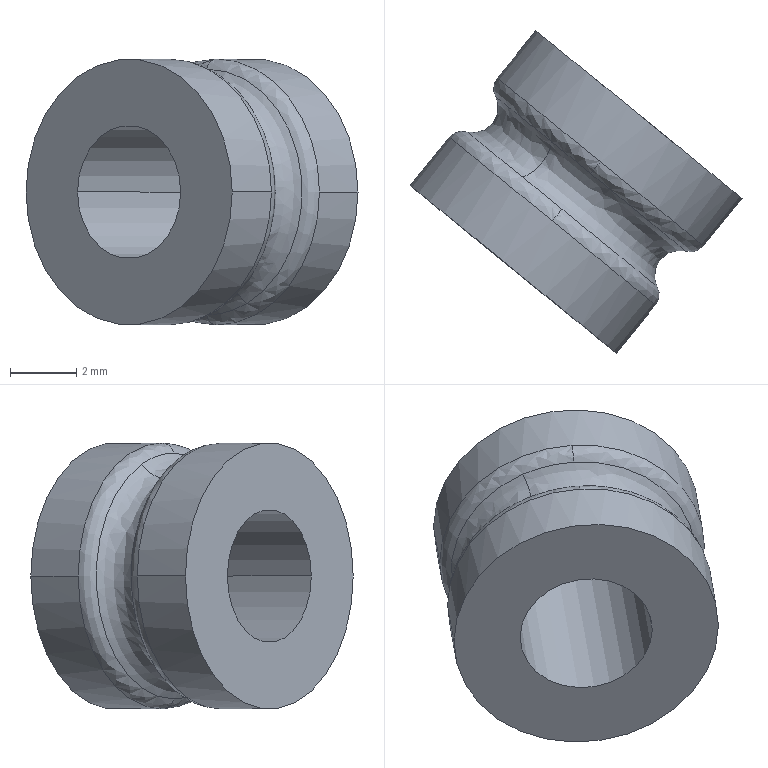Part | SolidWorks | features BaseBody 1 | 1 solid | 14 faces | box 9.992 x 9.702 x 8 mm | volume 204.482 mm3 | spline 6 | cylinder 6 | plane 2 | commonest cylinder face diameters 8 x4 4 x2
STEP:
#1=CARTESIAN_POINT('',(513.367,-138.193,327.178));
#2=VERTEX_POINT('',#1);
#3=CARTESIAN_POINT('',(512.175,-137.224,334.245));
#4=VERTEX_POINT('',#3);
#5=CARTESIAN_POINT('',(512.175,-137.224,330.545));
#6=DIRECTION('',(-0.6309,-0.7758,0.000000012));
#7=DIRECTION('',(-0.000000024,0.000000004,-1.));
#8=AXIS2_PLACEMENT_3D('',#5,#6,#7);
#9=CIRCLE('',#8,3.7);
#10=EDGE_CURVE('',#2,#4,#9,.T.);
#11=ORIENTED_EDGE('',*,*,#10,.T.);
#12=CARTESIAN_POINT('',(511.886,-137.58,334.545));
#13=VERTEX_POINT('',#12);
#14=CARTESIAN_POINT('',(511.886,-137.58,334.045));
#15=DIRECTION('',(0.7758,-0.6309,-0.000000021));
#16=DIRECTION('',(0.000000024,-0.000000004,1.));
#17=AXIS2_PLACEMENT_3D('',#14,#15,#16);
#18=CIRCLE('',#17,0.5);
#19=EDGE_CURVE('',#4,#13,#18,.T.);
#20=ORIENTED_EDGE('',*,*,#19,.T.);
#21=CARTESIAN_POINT('',(514.99,-140.104,330.545));
#22=VERTEX_POINT('',#21);
#23=CARTESIAN_POINT('',(511.886,-137.58,330.545));
#24=DIRECTION('',(-0.6309,-0.7758,0.000000012));
#25=DIRECTION('',(-0.7758,0.6309,0.));
#26=AXIS2_PLACEMENT_3D('',#23,#24,#25);
#27=CIRCLE('',#26,4.);
#28=EDGE_CURVE('',#22,#13,#27,.T.);
#29=ORIENTED_EDGE('',*,*,#28,.F.);
#30=CARTESIAN_POINT('',(511.886,-137.58,326.545));
#31=VERTEX_POINT('',#30);
#32=CARTESIAN_POINT('',(511.886,-137.58,330.545));
#33=DIRECTION('',(-0.6309,-0.7758,0.000000012));
#34=DIRECTION('',(-0.7758,0.6309,0.));
#35=AXIS2_PLACEMENT_3D('',#32,#33,#34);
#36=CIRCLE('',#35,4.);
#37=EDGE_CURVE('',#31,#22,#36,.T.);
#38=ORIENTED_EDGE('',*,*,#37,.F.);
#39=CARTESIAN_POINT('',(512.175,-137.224,326.845));
#40=VERTEX_POINT('',#39);
#41=CARTESIAN_POINT('',(511.886,-137.58,327.045));
#42=DIRECTION('',(-0.7758,0.6309,0.000000021));
#43=DIRECTION('',(-0.000000024,0.000000004,-1.));
#44=AXIS2_PLACEMENT_3D('',#41,#42,#43);
#45=CIRCLE('',#44,0.5);
#46=EDGE_CURVE('',#40,#31,#45,.T.);
#47=ORIENTED_EDGE('',*,*,#46,.F.);
#48=CARTESIAN_POINT('',(512.175,-137.224,330.545));
#49=DIRECTION('',(-0.6309,-0.7758,0.000000012));
#50=DIRECTION('',(-0.000000024,0.000000004,-1.));
#51=AXIS2_PLACEMENT_3D('',#48,#49,#50);
#52=CIRCLE('',#51,3.7);
#53=EDGE_CURVE('',#40,#2,#52,.T.);
#54=ORIENTED_EDGE('',*,*,#53,.T.);
#55=EDGE_LOOP('',(#11,#20,#29,#38,#47,#54));
#56=FACE_OUTER_BOUND('',#55,.T.);
#57=CARTESIAN_POINT('',(512.175,-137.224,334.245));
#58=CARTESIAN_POINT('',(517.917,-141.893,334.245));
#59=CARTESIAN_POINT('',(517.917,-141.893,326.845));
#60=CARTESIAN_POINT('',(512.175,-137.224,326.845));
#61=CARTESIAN_POINT('',(512.124,-137.288,334.432));
#62=CARTESIAN_POINT('',(518.156,-142.194,334.432));
#63=CARTESIAN_POINT('',(518.156,-142.194,326.657));
#64=CARTESIAN_POINT('',(512.124,-137.288,326.657));
#65=CARTESIAN_POINT('',(512.015,-137.421,334.545));
#66=CARTESIAN_POINT('',(518.222,-142.468,334.545));
#67=CARTESIAN_POINT('',(518.222,-142.468,326.545));
#68=CARTESIAN_POINT('',(512.015,-137.421,326.545));
#69=CARTESIAN_POINT('',(511.886,-137.58,334.545));
#70=CARTESIAN_POINT('',(518.093,-142.627,334.545));
#71=CARTESIAN_POINT('',(518.093,-142.627,326.545));
#72=CARTESIAN_POINT('',(511.886,-137.58,326.545));
#73=(BOUNDED_SURFACE()B_SPLINE_SURFACE(3,3,((#57,#58,#59,#60),(#61,#62,#63,#64),(#65,#66,#67,#68),(#69,#70,#71,#72)),.UNSPECIFIED.,.F.,.F.,.F.)B_SPLINE_SURFACE_WITH_KNOTS((4,4),(4,4),(0.,1.),(0.,1.),.UNSPECIFIED.)GEOMETRIC_REPRESENTATION_ITEM()RATIONAL_B_SPLINE_SURFACE(((1.,0.3333,0.3333,1.),(0.8911,0.297,0.297,0.8911),(0.8911,0.297,0.297,0.8911),(1.,0.3333,0.3333,1.)))REPRESENTATION_ITEM('')SURFACE());
#74=ADVANCED_FACE('',(#56),#73,.T.);
#75=CARTESIAN_POINT('',(514.234,-137.127,327.178));
#76=VERTEX_POINT('',#75);
#77=CARTESIAN_POINT('',(513.043,-136.158,326.845));
#78=VERTEX_POINT('',#77);
#79=CARTESIAN_POINT('',(513.043,-136.158,330.545));
#80=DIRECTION('',(0.6309,0.7758,-0.000000012));
#81=DIRECTION('',(0.000000024,-0.000000004,1.));
#82=AXIS2_PLACEMENT_3D('',#79,#80,#81);
#83=CIRCLE('',#82,3.7);
#84=EDGE_CURVE('',#76,#78,#83,.T.);
#85=ORIENTED_EDGE('',*,*,#84,.T.);
#86=CARTESIAN_POINT('',(513.332,-135.802,326.545));
#87=VERTEX_POINT('',#86);
#88=CARTESIAN_POINT('',(513.332,-135.802,327.045));
#89=DIRECTION('',(0.7758,-0.6309,-0.000000021));
#90=DIRECTION('',(-0.000000024,0.000000004,-1.));
#91=AXIS2_PLACEMENT_3D('',#88,#89,#90);
#92=CIRCLE('',#91,0.5);
#93=EDGE_CURVE('',#78,#87,#92,.T.);
#94=ORIENTED_EDGE('',*,*,#93,.T.);
#95=CARTESIAN_POINT('',(516.435,-138.326,330.545));
#96=VERTEX_POINT('',#95);
#97=CARTESIAN_POINT('',(513.332,-135.802,330.545));
#98=DIRECTION('',(0.6309,0.7758,-0.000000012));
#99=DIRECTION('',(-0.7758,0.6309,0.));
#100=AXIS2_PLACEMENT_3D('',#97,#98,#99);
#101=CIRCLE('',#100,4.);
#102=EDGE_CURVE('',#96,#87,#101,.T.);
#103=ORIENTED_EDGE('',*,*,#102,.F.);
#104=CARTESIAN_POINT('',(513.332,-135.802,334.545));
#105=VERTEX_POINT('',#104);
#106=CARTESIAN_POINT('',(513.332,-135.802,330.545));
#107=DIRECTION('',(0.6309,0.7758,-0.000000012));
#108=DIRECTION('',(-0.7758,0.6309,0.));
#109=AXIS2_PLACEMENT_3D('',#106,#107,#108);
#110=CIRCLE('',#109,4.);
#111=EDGE_CURVE('',#105,#96,#110,.T.);
#112=ORIENTED_EDGE('',*,*,#111,.F.);
#113=CARTESIAN_POINT('',(513.043,-136.158,334.245));
#114=VERTEX_POINT('',#113);
#115=CARTESIAN_POINT('',(513.332,-135.802,334.045));
#116=DIRECTION('',(-0.7758,0.6309,0.000000021));
#117=DIRECTION('',(0.000000024,-0.000000004,1.));
#118=AXIS2_PLACEMENT_3D('',#115,#116,#117);
#119=CIRCLE('',#118,0.5);
#120=EDGE_CURVE('',#114,#105,#119,.T.);
#121=ORIENTED_EDGE('',*,*,#120,.F.);
#122=CARTESIAN_POINT('',(513.043,-136.158,330.545));
#123=DIRECTION('',(0.6309,0.7758,-0.000000012));
#124=DIRECTION('',(0.000000024,-0.000000004,1.));
#125=AXIS2_PLACEMENT_3D('',#122,#123,#124);
#126=CIRCLE('',#125,3.7);
#127=EDGE_CURVE('',#114,#76,#126,.T.);
#128=ORIENTED_EDGE('',*,*,#127,.T.);
#129=EDGE_LOOP('',(#85,#94,#103,#112,#121,#128));
#130=FACE_OUTER_BOUND('',#129,.T.);
#131=CARTESIAN_POINT('',(513.043,-136.158,326.845));
#132=CARTESIAN_POINT('',(518.784,-140.827,326.845));
#133=CARTESIAN_POINT('',(518.784,-140.827,334.245));
#134=CARTESIAN_POINT('',(513.043,-136.158,334.245));
#135=CARTESIAN_POINT('',(513.094,-136.094,326.657));
#136=CARTESIAN_POINT('',(519.127,-141.,326.657));
#137=CARTESIAN_POINT('',(519.127,-141.,334.432));
#138=CARTESIAN_POINT('',(513.094,-136.094,334.432));
#139=CARTESIAN_POINT('',(513.203,-135.961,326.545));
#140=CARTESIAN_POINT('',(519.409,-141.009,326.545));
#141=CARTESIAN_POINT('',(519.409,-141.009,334.545));
#142=CARTESIAN_POINT('',(513.203,-135.961,334.545));
#143=CARTESIAN_POINT('',(513.332,-135.802,326.545));
#144=CARTESIAN_POINT('',(519.539,-140.85,326.545));
#145=CARTESIAN_POINT('',(519.539,-140.85,334.545));
#146=CARTESIAN_POINT('',(513.332,-135.802,334.545));
#147=(BOUNDED_SURFACE()B_SPLINE_SURFACE(3,3,((#131,#132,#133,#134),(#135,#136,#137,#138),(#139,#140,#141,#142),(#143,#144,#145,#146)),.UNSPECIFIED.,.F.,.F.,.F.)B_SPLINE_SURFACE_WITH_KNOTS((4,4),(4,4),(0.,1.),(0.,1.),.UNSPECIFIED.)GEOMETRIC_REPRESENTATION_ITEM()RATIONAL_B_SPLINE_SURFACE(((1.,0.3333,0.3333,1.),(0.8911,0.297,0.297,0.8911),(0.8911,0.297,0.297,0.8911),(1.,0.3333,0.3333,1.)))REPRESENTATION_ITEM('')SURFACE());
#148=ADVANCED_FACE('',(#130),#147,.T.);
#149=ORIENTED_EDGE('',*,*,#84,.F.);
#150=CARTESIAN_POINT('',(513.897,-137.739,326.905));
#151=DIRECTION('',(0.7058,-0.574,0.4151));
#152=DIRECTION('',(0.3221,-0.2619,-0.9098));
#153=AXIS2_PLACEMENT_3D('',#150,#151,#152);
#154=CIRCLE('',#153,0.75);
#155=EDGE_CURVE('',#76,#2,#154,.T.);
#156=ORIENTED_EDGE('',*,*,#155,.T.);
#157=ORIENTED_EDGE('',*,*,#53,.F.);
#158=CARTESIAN_POINT('',(510.984,-136.255,333.911));
#159=VERTEX_POINT('',#158);
#160=CARTESIAN_POINT('',(512.175,-137.224,330.545));
#161=DIRECTION('',(-0.6309,-0.7758,0.000000012));
#162=DIRECTION('',(-0.000000024,0.000000004,-1.));
#163=AXIS2_PLACEMENT_3D('',#160,#161,#162);
#164=CIRCLE('',#163,3.7);
#165=EDGE_CURVE('',#159,#40,#164,.T.);
#166=ORIENTED_EDGE('',*,*,#165,.F.);
#167=CARTESIAN_POINT('',(511.851,-135.189,333.911));
#168=VERTEX_POINT('',#167);
#169=CARTESIAN_POINT('',(511.321,-135.643,334.184));
#170=DIRECTION('',(-0.7058,0.574,-0.4151));
#171=DIRECTION('',(-0.3221,0.2619,0.9098));
#172=AXIS2_PLACEMENT_3D('',#169,#170,#171);
#173=CIRCLE('',#172,0.75);
#174=EDGE_CURVE('',#168,#159,#173,.T.);
#175=ORIENTED_EDGE('',*,*,#174,.F.);
#176=CARTESIAN_POINT('',(513.043,-136.158,330.545));
#177=DIRECTION('',(0.6309,0.7758,-0.000000012));
#178=DIRECTION('',(0.000000024,-0.000000004,1.));
#179=AXIS2_PLACEMENT_3D('',#176,#177,#178);
#180=CIRCLE('',#179,3.7);
#181=EDGE_CURVE('',#78,#168,#180,.T.);
#182=ORIENTED_EDGE('',*,*,#181,.F.);
#183=EDGE_LOOP('',(#149,#156,#157,#166,#175,#182));
#184=FACE_OUTER_BOUND('',#183,.T.);
#185=CARTESIAN_POINT('',(511.851,-135.189,333.911));
#186=CARTESIAN_POINT('',(506.628,-130.941,330.839));
#187=CARTESIAN_POINT('',(509.011,-132.879,324.106));
#188=CARTESIAN_POINT('',(514.234,-137.127,327.178));
#189=CARTESIAN_POINT('',(511.884,-135.609,333.274));
#190=CARTESIAN_POINT('',(507.649,-132.165,330.783));
#191=CARTESIAN_POINT('',(509.581,-133.736,325.324));
#192=CARTESIAN_POINT('',(513.816,-137.18,327.815));
#193=CARTESIAN_POINT('',(511.402,-136.202,333.274));
#194=CARTESIAN_POINT('',(507.167,-132.758,330.783));
#195=CARTESIAN_POINT('',(509.099,-134.329,325.324));
#196=CARTESIAN_POINT('',(513.334,-137.773,327.815));
#197=CARTESIAN_POINT('',(510.984,-136.255,333.911));
#198=CARTESIAN_POINT('',(505.761,-132.008,330.839));
#199=CARTESIAN_POINT('',(508.144,-133.946,324.106));
#200=CARTESIAN_POINT('',(513.367,-138.193,327.178));
#201=(BOUNDED_SURFACE()B_SPLINE_SURFACE(3,3,((#185,#186,#187,#188),(#189,#190,#191,#192),(#193,#194,#195,#196),(#197,#198,#199,#200)),.UNSPECIFIED.,.F.,.F.,.F.)B_SPLINE_SURFACE_WITH_KNOTS((4,4),(4,4),(0.,1.),(0.,1.),.UNSPECIFIED.)GEOMETRIC_REPRESENTATION_ITEM()RATIONAL_B_SPLINE_SURFACE(((1.,0.3333,0.3333,1.),(0.6,0.2,0.2,0.6),(0.6,0.2,0.2,0.6),(1.,0.3333,0.3333,1.)))REPRESENTATION_ITEM('')SURFACE());
#202=ADVANCED_FACE('',(#184),#201,.F.);
#203=CARTESIAN_POINT('',(512.258,-140.293,330.545));
#204=VERTEX_POINT('',#203);
#205=CARTESIAN_POINT('',(509.154,-137.769,330.545));
#206=VERTEX_POINT('',#205);
#207=CARTESIAN_POINT('',(510.706,-139.031,330.545));
#208=DIRECTION('',(0.6309,0.7758,-0.000000012));
#209=DIRECTION('',(-0.7758,0.6309,0.));
#210=AXIS2_PLACEMENT_3D('',#207,#208,#209);
#211=CIRCLE('',#210,2.);
#212=EDGE_CURVE('',#204,#206,#211,.T.);
#213=ORIENTED_EDGE('',*,*,#212,.F.);
#214=CARTESIAN_POINT('',(516.043,-135.638,330.545));
#215=VERTEX_POINT('',#214);
#216=CARTESIAN_POINT('',(516.043,-135.638,330.545));
#217=DIRECTION('',(0.6309,0.7758,-0.000000012));
#218=VECTOR('',#217,1000.);
#219=LINE('',#216,#218);
#220=EDGE_CURVE('',#204,#215,#219,.T.);
#221=ORIENTED_EDGE('',*,*,#220,.T.);
#222=CARTESIAN_POINT('',(512.94,-133.114,330.545));
#223=VERTEX_POINT('',#222);
#224=CARTESIAN_POINT('',(514.492,-134.376,330.545));
#225=DIRECTION('',(-0.6309,-0.7758,0.000000012));
#226=DIRECTION('',(-0.7758,0.6309,0.));
#227=AXIS2_PLACEMENT_3D('',#224,#225,#226);
#228=CIRCLE('',#227,2.);
#229=EDGE_CURVE('',#223,#215,#228,.T.);
#230=ORIENTED_EDGE('',*,*,#229,.F.);
#231=CARTESIAN_POINT('',(512.94,-133.114,330.545));
#232=DIRECTION('',(0.6309,0.7758,-0.000000012));
#233=VECTOR('',#232,1000.);
#234=LINE('',#231,#233);
#235=EDGE_CURVE('',#206,#223,#234,.T.);
#236=ORIENTED_EDGE('',*,*,#235,.F.);
#237=EDGE_LOOP('',(#213,#221,#230,#236));
#238=FACE_OUTER_BOUND('',#237,.T.);
#239=CARTESIAN_POINT('',(514.492,-134.376,330.545));
#240=DIRECTION('',(0.6309,0.7758,-0.000000012));
#241=DIRECTION('',(-0.7758,0.6309,0.));
#242=AXIS2_PLACEMENT_3D('',#239,#240,#241);
#243=CYLINDRICAL_SURFACE('',#242,2.);
#244=ADVANCED_FACE('',(#238),#243,.F.);
#245=CARTESIAN_POINT('',(507.603,-136.507,330.545));
#246=VERTEX_POINT('',#245);
#247=CARTESIAN_POINT('',(513.809,-141.555,330.545));
#248=VERTEX_POINT('',#247);
#249=CARTESIAN_POINT('',(510.706,-139.031,330.545));
#250=DIRECTION('',(0.6309,0.7758,-0.000000012));
#251=DIRECTION('',(-0.7758,0.6309,0.));
#252=AXIS2_PLACEMENT_3D('',#249,#250,#251);
#253=CIRCLE('',#252,4.);
#254=EDGE_CURVE('',#246,#248,#253,.T.);
#255=ORIENTED_EDGE('',*,*,#254,.T.);
#256=CARTESIAN_POINT('',(513.809,-141.555,330.545));
#257=DIRECTION('',(0.6309,0.7758,-0.000000012));
#258=VECTOR('',#257,1000.);
#259=LINE('',#256,#258);
#260=EDGE_CURVE('',#248,#22,#259,.T.);
#261=ORIENTED_EDGE('',*,*,#260,.T.);
#262=ORIENTED_EDGE('',*,*,#28,.T.);
#263=CARTESIAN_POINT('',(508.783,-135.056,330.545));
#264=VERTEX_POINT('',#263);
#265=CARTESIAN_POINT('',(511.886,-137.58,330.545));
#266=DIRECTION('',(-0.6309,-0.7758,0.000000012));
#267=DIRECTION('',(-0.7758,0.6309,0.));
#268=AXIS2_PLACEMENT_3D('',#265,#266,#267);
#269=CIRCLE('',#268,4.);
#270=EDGE_CURVE('',#13,#264,#269,.T.);
#271=ORIENTED_EDGE('',*,*,#270,.T.);
#272=CARTESIAN_POINT('',(507.603,-136.507,330.545));
#273=DIRECTION('',(0.6309,0.7758,-0.000000012));
#274=VECTOR('',#273,1000.);
#275=LINE('',#272,#274);
#276=EDGE_CURVE('',#246,#264,#275,.T.);
#277=ORIENTED_EDGE('',*,*,#276,.F.);
#278=EDGE_LOOP('',(#255,#261,#262,#271,#277));
#279=FACE_OUTER_BOUND('',#278,.T.);
#280=CARTESIAN_POINT('',(510.706,-139.031,330.545));
#281=DIRECTION('',(0.6309,0.7758,-0.000000012));
#282=DIRECTION('',(-0.7758,0.6309,0.));
#283=AXIS2_PLACEMENT_3D('',#280,#281,#282);
#284=CYLINDRICAL_SURFACE('',#283,4.);
#285=ADVANCED_FACE('',(#279),#284,.T.);
#286=CARTESIAN_POINT('',(510.228,-133.278,330.545));
#287=VERTEX_POINT('',#286);
#288=CARTESIAN_POINT('',(513.332,-135.802,330.545));
#289=DIRECTION('',(0.6309,0.7758,-0.000000012));
#290=DIRECTION('',(-0.7758,0.6309,0.));
#291=AXIS2_PLACEMENT_3D('',#288,#289,#290);
#292=CIRCLE('',#291,4.);
#293=EDGE_CURVE('',#287,#105,#292,.T.);
#294=ORIENTED_EDGE('',*,*,#293,.T.);
#295=ORIENTED_EDGE('',*,*,#111,.T.);
#296=CARTESIAN_POINT('',(517.595,-136.9,330.545));
#297=VERTEX_POINT('',#296);
#298=CARTESIAN_POINT('',(513.809,-141.555,330.545));
#299=DIRECTION('',(0.6309,0.7758,-0.000000012));
#300=VECTOR('',#299,1000.);
#301=LINE('',#298,#300);
#302=EDGE_CURVE('',#96,#297,#301,.T.);
#303=ORIENTED_EDGE('',*,*,#302,.T.);
#304=CARTESIAN_POINT('',(511.388,-131.852,330.545));
#305=VERTEX_POINT('',#304);
#306=CARTESIAN_POINT('',(514.492,-134.376,330.545));
#307=DIRECTION('',(0.6309,0.7758,-0.000000012));
#308=DIRECTION('',(-0.7758,0.6309,0.));
#309=AXIS2_PLACEMENT_3D('',#306,#307,#308);
#310=CIRCLE('',#309,4.);
#311=EDGE_CURVE('',#305,#297,#310,.T.);
#312=ORIENTED_EDGE('',*,*,#311,.F.);
#313=CARTESIAN_POINT('',(507.603,-136.507,330.545));
#314=DIRECTION('',(0.6309,0.7758,-0.000000012));
#315=VECTOR('',#314,1000.);
#316=LINE('',#313,#315);
#317=EDGE_CURVE('',#287,#305,#316,.T.);
#318=ORIENTED_EDGE('',*,*,#317,.F.);
#319=EDGE_LOOP('',(#294,#295,#303,#312,#318));
#320=FACE_OUTER_BOUND('',#319,.T.);
#321=CARTESIAN_POINT('',(510.706,-139.031,330.545));
#322=DIRECTION('',(0.6309,0.7758,-0.000000012));
#323=DIRECTION('',(-0.7758,0.6309,0.));
#324=AXIS2_PLACEMENT_3D('',#321,#322,#323);
#325=CYLINDRICAL_SURFACE('',#324,4.);
#326=ADVANCED_FACE('',(#320),#325,.T.);
#327=ORIENTED_EDGE('',*,*,#220,.F.);
#328=CARTESIAN_POINT('',(510.706,-139.031,330.545));
#329=DIRECTION('',(0.6309,0.7758,-0.000000012));
#330=DIRECTION('',(-0.7758,0.6309,0.));
#331=AXIS2_PLACEMENT_3D('',#328,#329,#330);
#332=CIRCLE('',#331,2.);
#333=EDGE_CURVE('',#206,#204,#332,.T.);
#334=ORIENTED_EDGE('',*,*,#333,.F.);
#335=ORIENTED_EDGE('',*,*,#235,.T.);
#336=CARTESIAN_POINT('',(514.492,-134.376,330.545));
#337=DIRECTION('',(-0.6309,-0.7758,0.000000012));
#338=DIRECTION('',(-0.7758,0.6309,0.));
#339=AXIS2_PLACEMENT_3D('',#336,#337,#338);
#340=CIRCLE('',#339,2.);
#341=EDGE_CURVE('',#215,#223,#340,.T.);
#342=ORIENTED_EDGE('',*,*,#341,.F.);
#343=EDGE_LOOP('',(#327,#334,#335,#342));
#344=FACE_OUTER_BOUND('',#343,.T.);
#345=CARTESIAN_POINT('',(514.492,-134.376,330.545));
#346=DIRECTION('',(0.6309,0.7758,-0.000000012));
#347=DIRECTION('',(-0.7758,0.6309,0.));
#348=AXIS2_PLACEMENT_3D('',#345,#346,#347);
#349=CYLINDRICAL_SURFACE('',#348,2.);
#350=ADVANCED_FACE('',(#344),#349,.F.);
#351=ORIENTED_EDGE('',*,*,#254,.F.);
#352=CARTESIAN_POINT('',(510.706,-139.031,330.545));
#353=DIRECTION('',(0.6309,0.7758,-0.000000012));
#354=DIRECTION('',(-0.7758,0.6309,0.));
#355=AXIS2_PLACEMENT_3D('',#352,#353,#354);
#356=CIRCLE('',#355,4.);
#357=EDGE_CURVE('',#248,#246,#356,.T.);
#358=ORIENTED_EDGE('',*,*,#357,.F.);
#359=EDGE_LOOP('',(#351,#358));
#360=FACE_OUTER_BOUND('',#359,.T.);
#361=ORIENTED_EDGE('',*,*,#333,.T.);
#362=ORIENTED_EDGE('',*,*,#212,.T.);
#363=EDGE_LOOP('',(#361,#362));
#364=FACE_BOUND('',#363,.T.);
#365=CARTESIAN_POINT('',(510.706,-139.031,330.545));
#366=DIRECTION('',(0.6309,0.7758,-0.000000012));
#367=DIRECTION('',(-0.7758,0.6309,0.));
#368=AXIS2_PLACEMENT_3D('',#365,#366,#367);
#369=PLANE('',#368);
#370=ADVANCED_FACE('',(#360,#364),#369,.F.);
#371=ORIENTED_EDGE('',*,*,#311,.T.);
#372=CARTESIAN_POINT('',(514.492,-134.376,330.545));
#373=DIRECTION('',(0.6309,0.7758,-0.000000012));
#374=DIRECTION('',(-0.7758,0.6309,0.));
#375=AXIS2_PLACEMENT_3D('',#372,#373,#374);
#376=CIRCLE('',#375,4.);
#377=EDGE_CURVE('',#297,#305,#376,.T.);
#378=ORIENTED_EDGE('',*,*,#377,.T.);
#379=EDGE_LOOP('',(#371,#378));
#380=FACE_OUTER_BOUND('',#379,.T.);
#381=ORIENTED_EDGE('',*,*,#229,.T.);
#382=ORIENTED_EDGE('',*,*,#341,.T.);
#383=EDGE_LOOP('',(#381,#382));
#384=FACE_BOUND('',#383,.T.);
#385=CARTESIAN_POINT('',(514.492,-134.376,330.545));
#386=DIRECTION('',(0.6309,0.7758,-0.000000012));
#387=DIRECTION('',(-0.7758,0.6309,0.));
#388=AXIS2_PLACEMENT_3D('',#385,#386,#387);
#389=PLANE('',#388);
#390=ADVANCED_FACE('',(#380,#384),#389,.T.);
#391=ORIENTED_EDGE('',*,*,#260,.F.);
#392=ORIENTED_EDGE('',*,*,#357,.T.);
#393=ORIENTED_EDGE('',*,*,#276,.T.);
#394=CARTESIAN_POINT('',(511.886,-137.58,330.545));
#395=DIRECTION('',(-0.6309,-0.7758,0.000000012));
#396=DIRECTION('',(-0.7758,0.6309,0.));
#397=AXIS2_PLACEMENT_3D('',#394,#395,#396);
#398=CIRCLE('',#397,4.);
#399=EDGE_CURVE('',#264,#31,#398,.T.);
#400=ORIENTED_EDGE('',*,*,#399,.T.);
#401=ORIENTED_EDGE('',*,*,#37,.T.);
#402=EDGE_LOOP('',(#391,#392,#393,#400,#401));
#403=FACE_OUTER_BOUND('',#402,.T.);
#404=CARTESIAN_POINT('',(510.706,-139.031,330.545));
#405=DIRECTION('',(0.6309,0.7758,-0.000000012));
#406=DIRECTION('',(-0.7758,0.6309,0.));
#407=AXIS2_PLACEMENT_3D('',#404,#405,#406);
#408=CYLINDRICAL_SURFACE('',#407,4.);
#409=ADVANCED_FACE('',(#403),#408,.T.);
#410=ORIENTED_EDGE('',*,*,#302,.F.);
#411=ORIENTED_EDGE('',*,*,#102,.T.);
#412=CARTESIAN_POINT('',(513.332,-135.802,330.545));
#413=DIRECTION('',(0.6309,0.7758,-0.000000012));
#414=DIRECTION('',(-0.7758,0.6309,0.));
#415=AXIS2_PLACEMENT_3D('',#412,#413,#414);
#416=CIRCLE('',#415,4.);
#417=EDGE_CURVE('',#87,#287,#416,.T.);
#418=ORIENTED_EDGE('',*,*,#417,.T.);
#419=ORIENTED_EDGE('',*,*,#317,.T.);
#420=ORIENTED_EDGE('',*,*,#377,.F.);
#421=EDGE_LOOP('',(#410,#411,#418,#419,#420));
#422=FACE_OUTER_BOUND('',#421,.T.);
#423=CARTESIAN_POINT('',(510.706,-139.031,330.545));
#424=DIRECTION('',(0.6309,0.7758,-0.000000012));
#425=DIRECTION('',(-0.7758,0.6309,0.));
#426=AXIS2_PLACEMENT_3D('',#423,#424,#425);
#427=CYLINDRICAL_SURFACE('',#426,4.);
#428=ADVANCED_FACE('',(#422),#427,.T.);
#429=ORIENTED_EDGE('',*,*,#19,.F.);
#430=CARTESIAN_POINT('',(512.175,-137.224,330.545));
#431=DIRECTION('',(-0.6309,-0.7758,0.000000012));
#432=DIRECTION('',(-0.000000024,0.000000004,-1.));
#433=AXIS2_PLACEMENT_3D('',#430,#431,#432);
#434=CIRCLE('',#433,3.7);
#435=EDGE_CURVE('',#4,#159,#434,.T.);
#436=ORIENTED_EDGE('',*,*,#435,.T.);
#437=ORIENTED_EDGE('',*,*,#165,.T.);
#438=ORIENTED_EDGE('',*,*,#46,.T.);
#439=ORIENTED_EDGE('',*,*,#399,.F.);
#440=ORIENTED_EDGE('',*,*,#270,.F.);
#441=EDGE_LOOP('',(#429,#436,#437,#438,#439,#440));
#442=FACE_OUTER_BOUND('',#441,.T.);
#443=CARTESIAN_POINT('',(512.175,-137.224,326.845));
#444=CARTESIAN_POINT('',(506.434,-132.555,326.845));
#445=CARTESIAN_POINT('',(506.434,-132.555,334.245));
#446=CARTESIAN_POINT('',(512.175,-137.224,334.245));
#447=CARTESIAN_POINT('',(512.124,-137.288,326.657));
#448=CARTESIAN_POINT('',(506.091,-132.382,326.657));
#449=CARTESIAN_POINT('',(506.091,-132.382,334.432));
#450=CARTESIAN_POINT('',(512.124,-137.288,334.432));
#451=CARTESIAN_POINT('',(512.015,-137.421,326.545));
#452=CARTESIAN_POINT('',(505.809,-132.373,326.545));
#453=CARTESIAN_POINT('',(505.809,-132.373,334.545));
#454=CARTESIAN_POINT('',(512.015,-137.421,334.545));
#455=CARTESIAN_POINT('',(511.886,-137.58,326.545));
#456=CARTESIAN_POINT('',(505.679,-132.532,326.545));
#457=CARTESIAN_POINT('',(505.679,-132.532,334.545));
#458=CARTESIAN_POINT('',(511.886,-137.58,334.545));
#459=(BOUNDED_SURFACE()B_SPLINE_SURFACE(3,3,((#443,#444,#445,#446),(#447,#448,#449,#450),(#451,#452,#453,#454),(#455,#456,#457,#458)),.UNSPECIFIED.,.F.,.F.,.F.)B_SPLINE_SURFACE_WITH_KNOTS((4,4),(4,4),(0.,1.),(0.,1.),.UNSPECIFIED.)GEOMETRIC_REPRESENTATION_ITEM()RATIONAL_B_SPLINE_SURFACE(((1.,0.3333,0.3333,1.),(0.8911,0.297,0.297,0.8911),(0.8911,0.297,0.297,0.8911),(1.,0.3333,0.3333,1.)))REPRESENTATION_ITEM('')SURFACE());
#460=ADVANCED_FACE('',(#442),#459,.T.);
#461=ORIENTED_EDGE('',*,*,#93,.F.);
#462=ORIENTED_EDGE('',*,*,#181,.T.);
#463=CARTESIAN_POINT('',(513.043,-136.158,330.545));
#464=DIRECTION('',(0.6309,0.7758,-0.000000012));
#465=DIRECTION('',(0.000000024,-0.000000004,1.));
#466=AXIS2_PLACEMENT_3D('',#463,#464,#465);
#467=CIRCLE('',#466,3.7);
#468=EDGE_CURVE('',#168,#114,#467,.T.);
#469=ORIENTED_EDGE('',*,*,#468,.T.);
#470=ORIENTED_EDGE('',*,*,#120,.T.);
#471=ORIENTED_EDGE('',*,*,#293,.F.);
#472=ORIENTED_EDGE('',*,*,#417,.F.);
#473=EDGE_LOOP('',(#461,#462,#469,#470,#471,#472));
#474=FACE_OUTER_BOUND('',#473,.T.);
#475=CARTESIAN_POINT('',(513.043,-136.158,334.245));
#476=CARTESIAN_POINT('',(507.302,-131.489,334.245));
#477=CARTESIAN_POINT('',(507.302,-131.489,326.845));
#478=CARTESIAN_POINT('',(513.043,-136.158,326.845));
#479=CARTESIAN_POINT('',(513.094,-136.094,334.432));
#480=CARTESIAN_POINT('',(507.062,-131.188,334.432));
#481=CARTESIAN_POINT('',(507.062,-131.188,326.657));
#482=CARTESIAN_POINT('',(513.094,-136.094,326.657));
#483=CARTESIAN_POINT('',(513.203,-135.961,334.545));
#484=CARTESIAN_POINT('',(506.996,-130.914,334.545));
#485=CARTESIAN_POINT('',(506.996,-130.914,326.545));
#486=CARTESIAN_POINT('',(513.203,-135.961,326.545));
#487=CARTESIAN_POINT('',(513.332,-135.802,334.545));
#488=CARTESIAN_POINT('',(507.125,-130.755,334.545));
#489=CARTESIAN_POINT('',(507.125,-130.755,326.545));
#490=CARTESIAN_POINT('',(513.332,-135.802,326.545));
#491=(BOUNDED_SURFACE()B_SPLINE_SURFACE(3,3,((#475,#476,#477,#478),(#479,#480,#481,#482),(#483,#484,#485,#486),(#487,#488,#489,#490)),.UNSPECIFIED.,.F.,.F.,.F.)B_SPLINE_SURFACE_WITH_KNOTS((4,4),(4,4),(0.,1.),(0.,1.),.UNSPECIFIED.)GEOMETRIC_REPRESENTATION_ITEM()RATIONAL_B_SPLINE_SURFACE(((1.,0.3333,0.3333,1.),(0.8911,0.297,0.297,0.8911),(0.8911,0.297,0.297,0.8911),(1.,0.3333,0.3333,1.)))REPRESENTATION_ITEM('')SURFACE());
#492=ADVANCED_FACE('',(#474),#491,.T.);
#493=ORIENTED_EDGE('',*,*,#155,.F.);
#494=ORIENTED_EDGE('',*,*,#127,.F.);
#495=ORIENTED_EDGE('',*,*,#468,.F.);
#496=ORIENTED_EDGE('',*,*,#174,.T.);
#497=ORIENTED_EDGE('',*,*,#435,.F.);
#498=ORIENTED_EDGE('',*,*,#10,.F.);
#499=EDGE_LOOP('',(#493,#494,#495,#496,#497,#498));
#500=FACE_OUTER_BOUND('',#499,.T.);
#501=CARTESIAN_POINT('',(514.234,-137.127,327.178));
#502=CARTESIAN_POINT('',(519.458,-141.374,330.25));
#503=CARTESIAN_POINT('',(517.074,-139.436,336.983));
#504=CARTESIAN_POINT('',(511.851,-135.189,333.911));
#505=CARTESIAN_POINT('',(513.816,-137.18,327.815));
#506=CARTESIAN_POINT('',(518.051,-140.624,330.306));
#507=CARTESIAN_POINT('',(516.119,-139.053,335.765));
#508=CARTESIAN_POINT('',(511.884,-135.609,333.274));
#509=CARTESIAN_POINT('',(513.334,-137.773,327.815));
#510=CARTESIAN_POINT('',(517.569,-141.217,330.306));
#511=CARTESIAN_POINT('',(515.637,-139.646,335.765));
#512=CARTESIAN_POINT('',(511.402,-136.202,333.274));
#513=CARTESIAN_POINT('',(513.367,-138.193,327.178));
#514=CARTESIAN_POINT('',(518.59,-142.441,330.25));
#515=CARTESIAN_POINT('',(516.207,-140.503,336.983));
#516=CARTESIAN_POINT('',(510.984,-136.255,333.911));
#517=(BOUNDED_SURFACE()B_SPLINE_SURFACE(3,3,((#501,#502,#503,#504),(#505,#506,#507,#508),(#509,#510,#511,#512),(#513,#514,#515,#516)),.UNSPECIFIED.,.F.,.F.,.F.)B_SPLINE_SURFACE_WITH_KNOTS((4,4),(4,4),(0.,1.),(0.,1.),.UNSPECIFIED.)GEOMETRIC_REPRESENTATION_ITEM()RATIONAL_B_SPLINE_SURFACE(((1.,0.3333,0.3333,1.),(0.6,0.2,0.2,0.6),(0.6,0.2,0.2,0.6),(1.,0.3333,0.3333,1.)))REPRESENTATION_ITEM('')SURFACE());
#518=ADVANCED_FACE('',(#500),#517,.F.);
#519=CLOSED_SHELL('',(#74,#148,#202,#244,#285,#326,#350,#370,#390,#409,#428,#460,#492,#518));
#520=MANIFOLD_SOLID_BREP('',#519);
#521=CARTESIAN_POINT('',(0.,0.,0.));
#522=DIRECTION('',(0.,0.,1.));
#523=DIRECTION('',(1.,0.,0.));
#524=AXIS2_PLACEMENT_3D('',#521,#522,#523);
#525=(LENGTH_UNIT()NAMED_UNIT(*)SI_UNIT(.MILLI.,.METRE.));
#526=UNCERTAINTY_MEASURE_WITH_UNIT(LENGTH_MEASURE(0.00001),#525,'','');
#527=(NAMED_UNIT(*)PLANE_ANGLE_UNIT()SI_UNIT($,.RADIAN.));
#528=(NAMED_UNIT(*)SI_UNIT($,.STERADIAN.)SOLID_ANGLE_UNIT());
#529=(GEOMETRIC_REPRESENTATION_CONTEXT(3)GLOBAL_UNCERTAINTY_ASSIGNED_CONTEXT((#526))GLOBAL_UNIT_ASSIGNED_CONTEXT((#525,#527,#528))REPRESENTATION_CONTEXT('',''));
#530=ADVANCED_BREP_SHAPE_REPRESENTATION('',(#520,#524),#529);